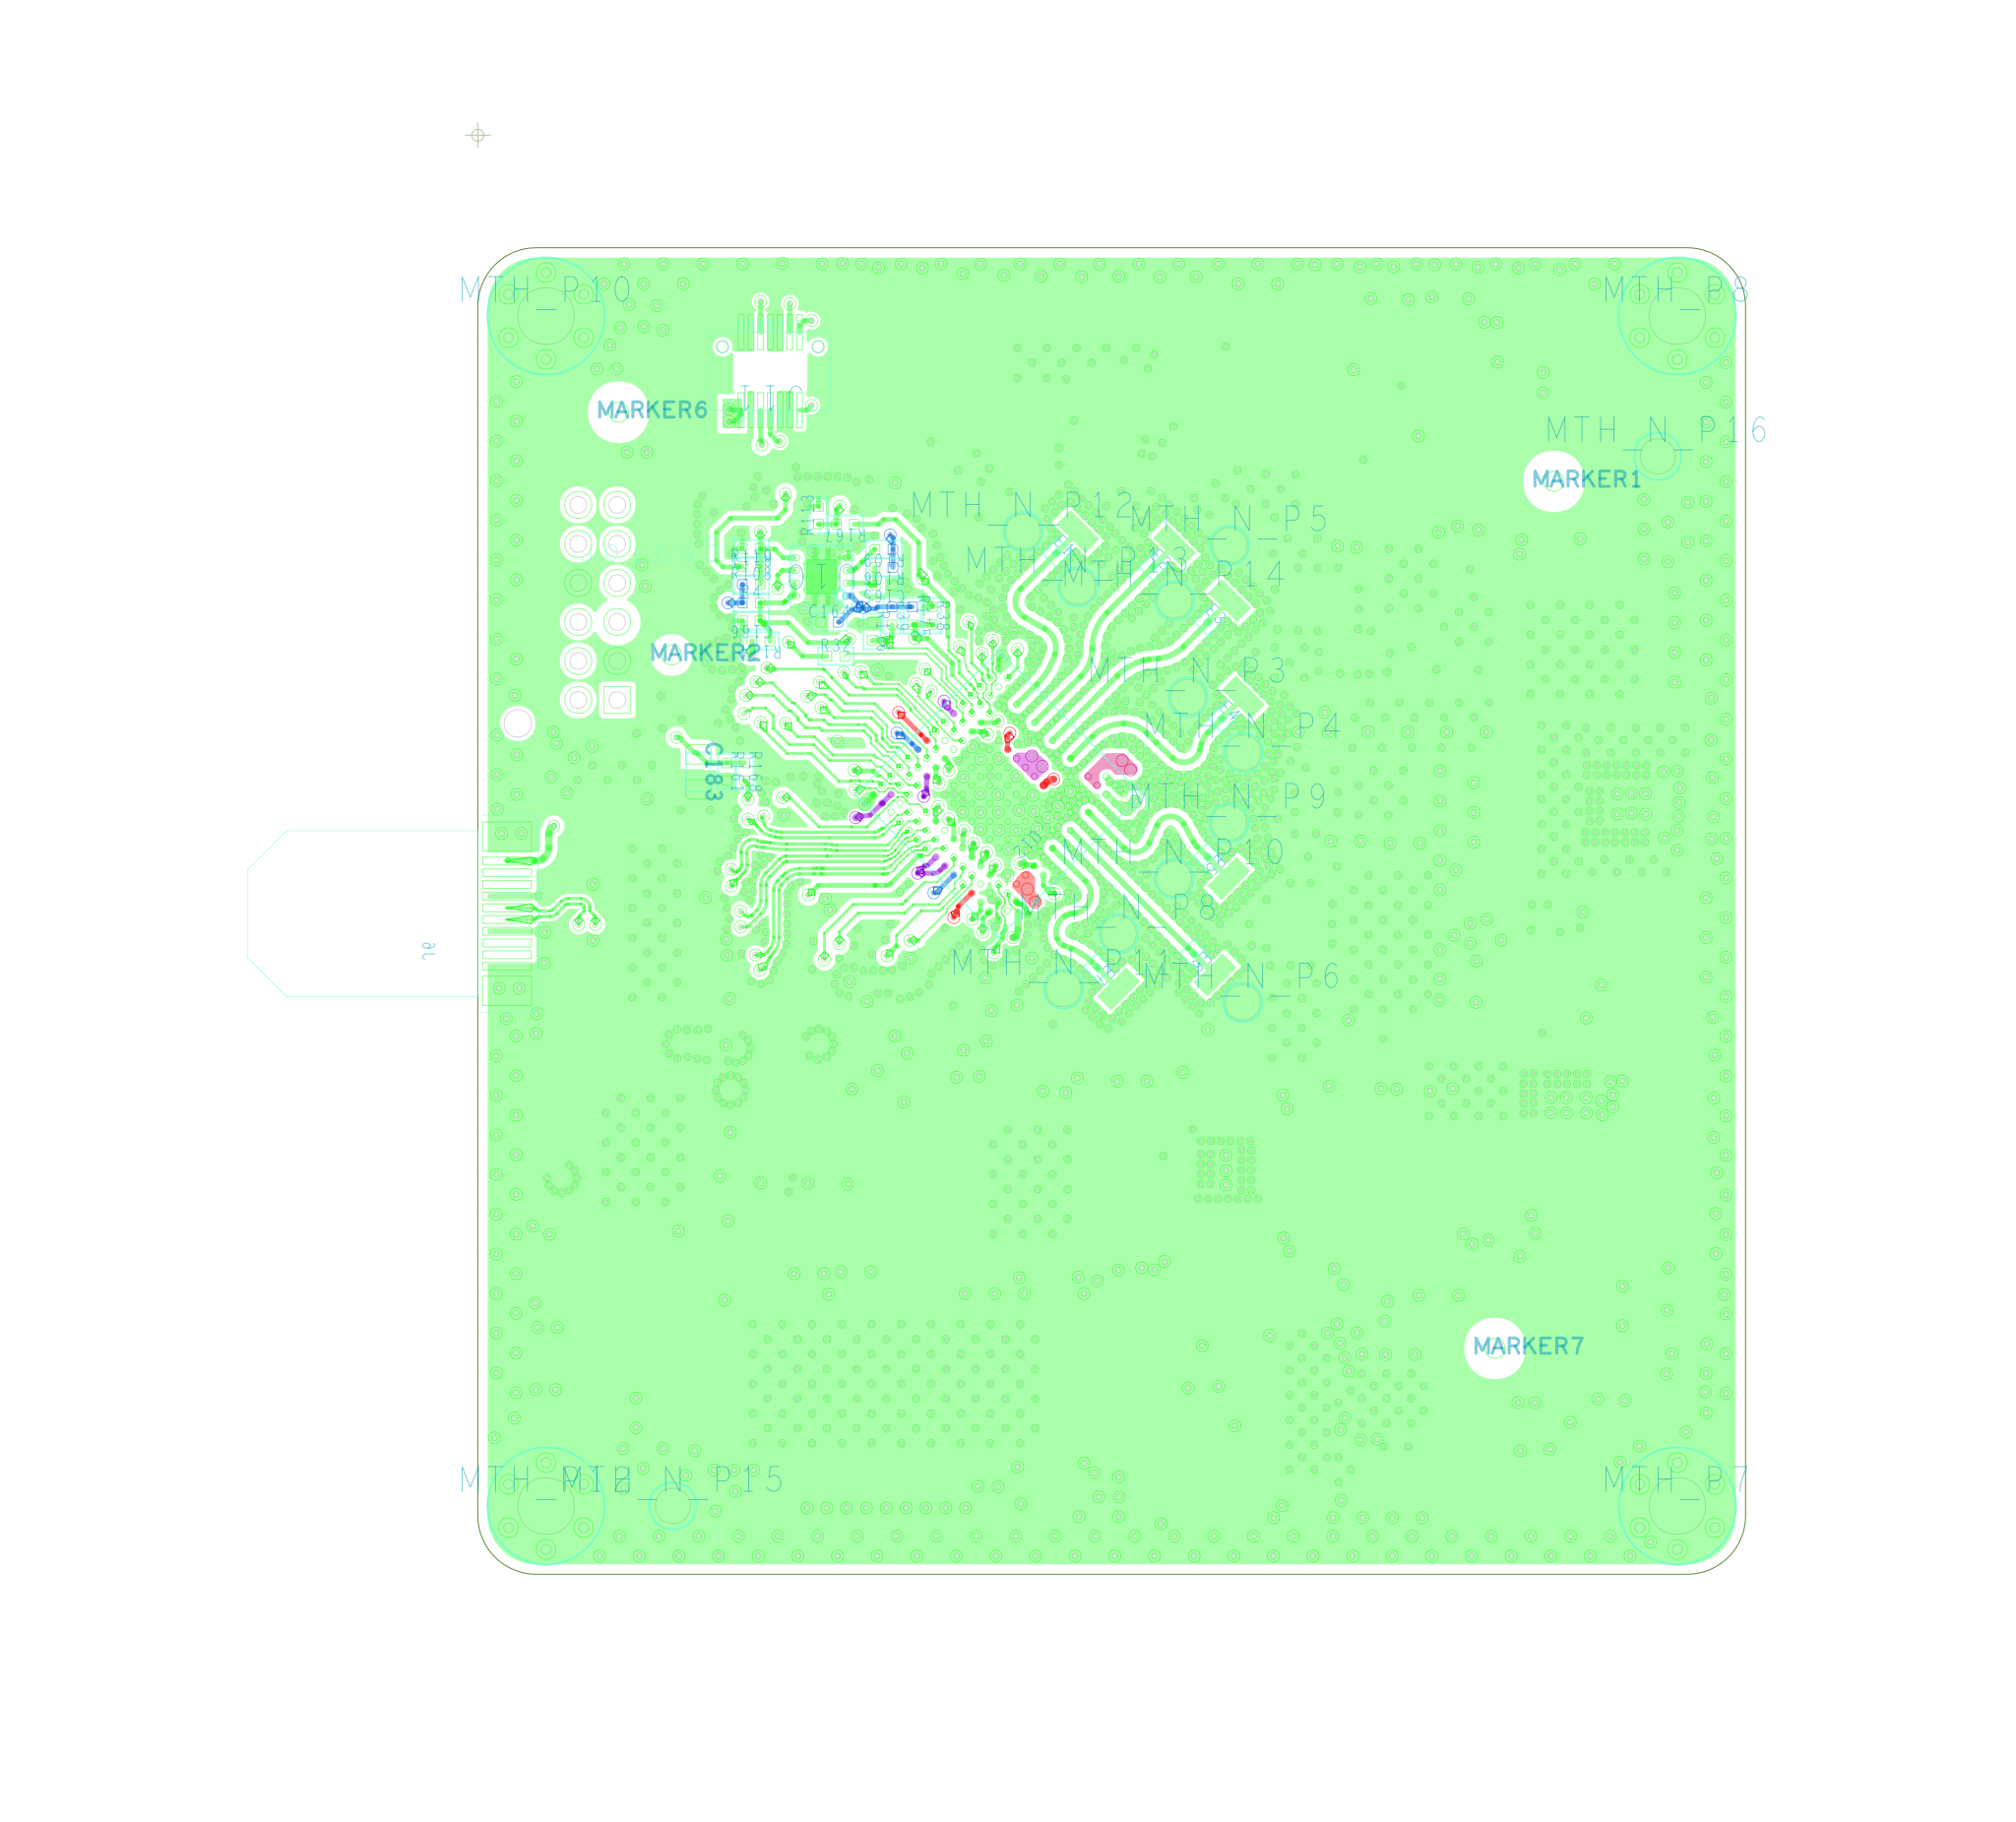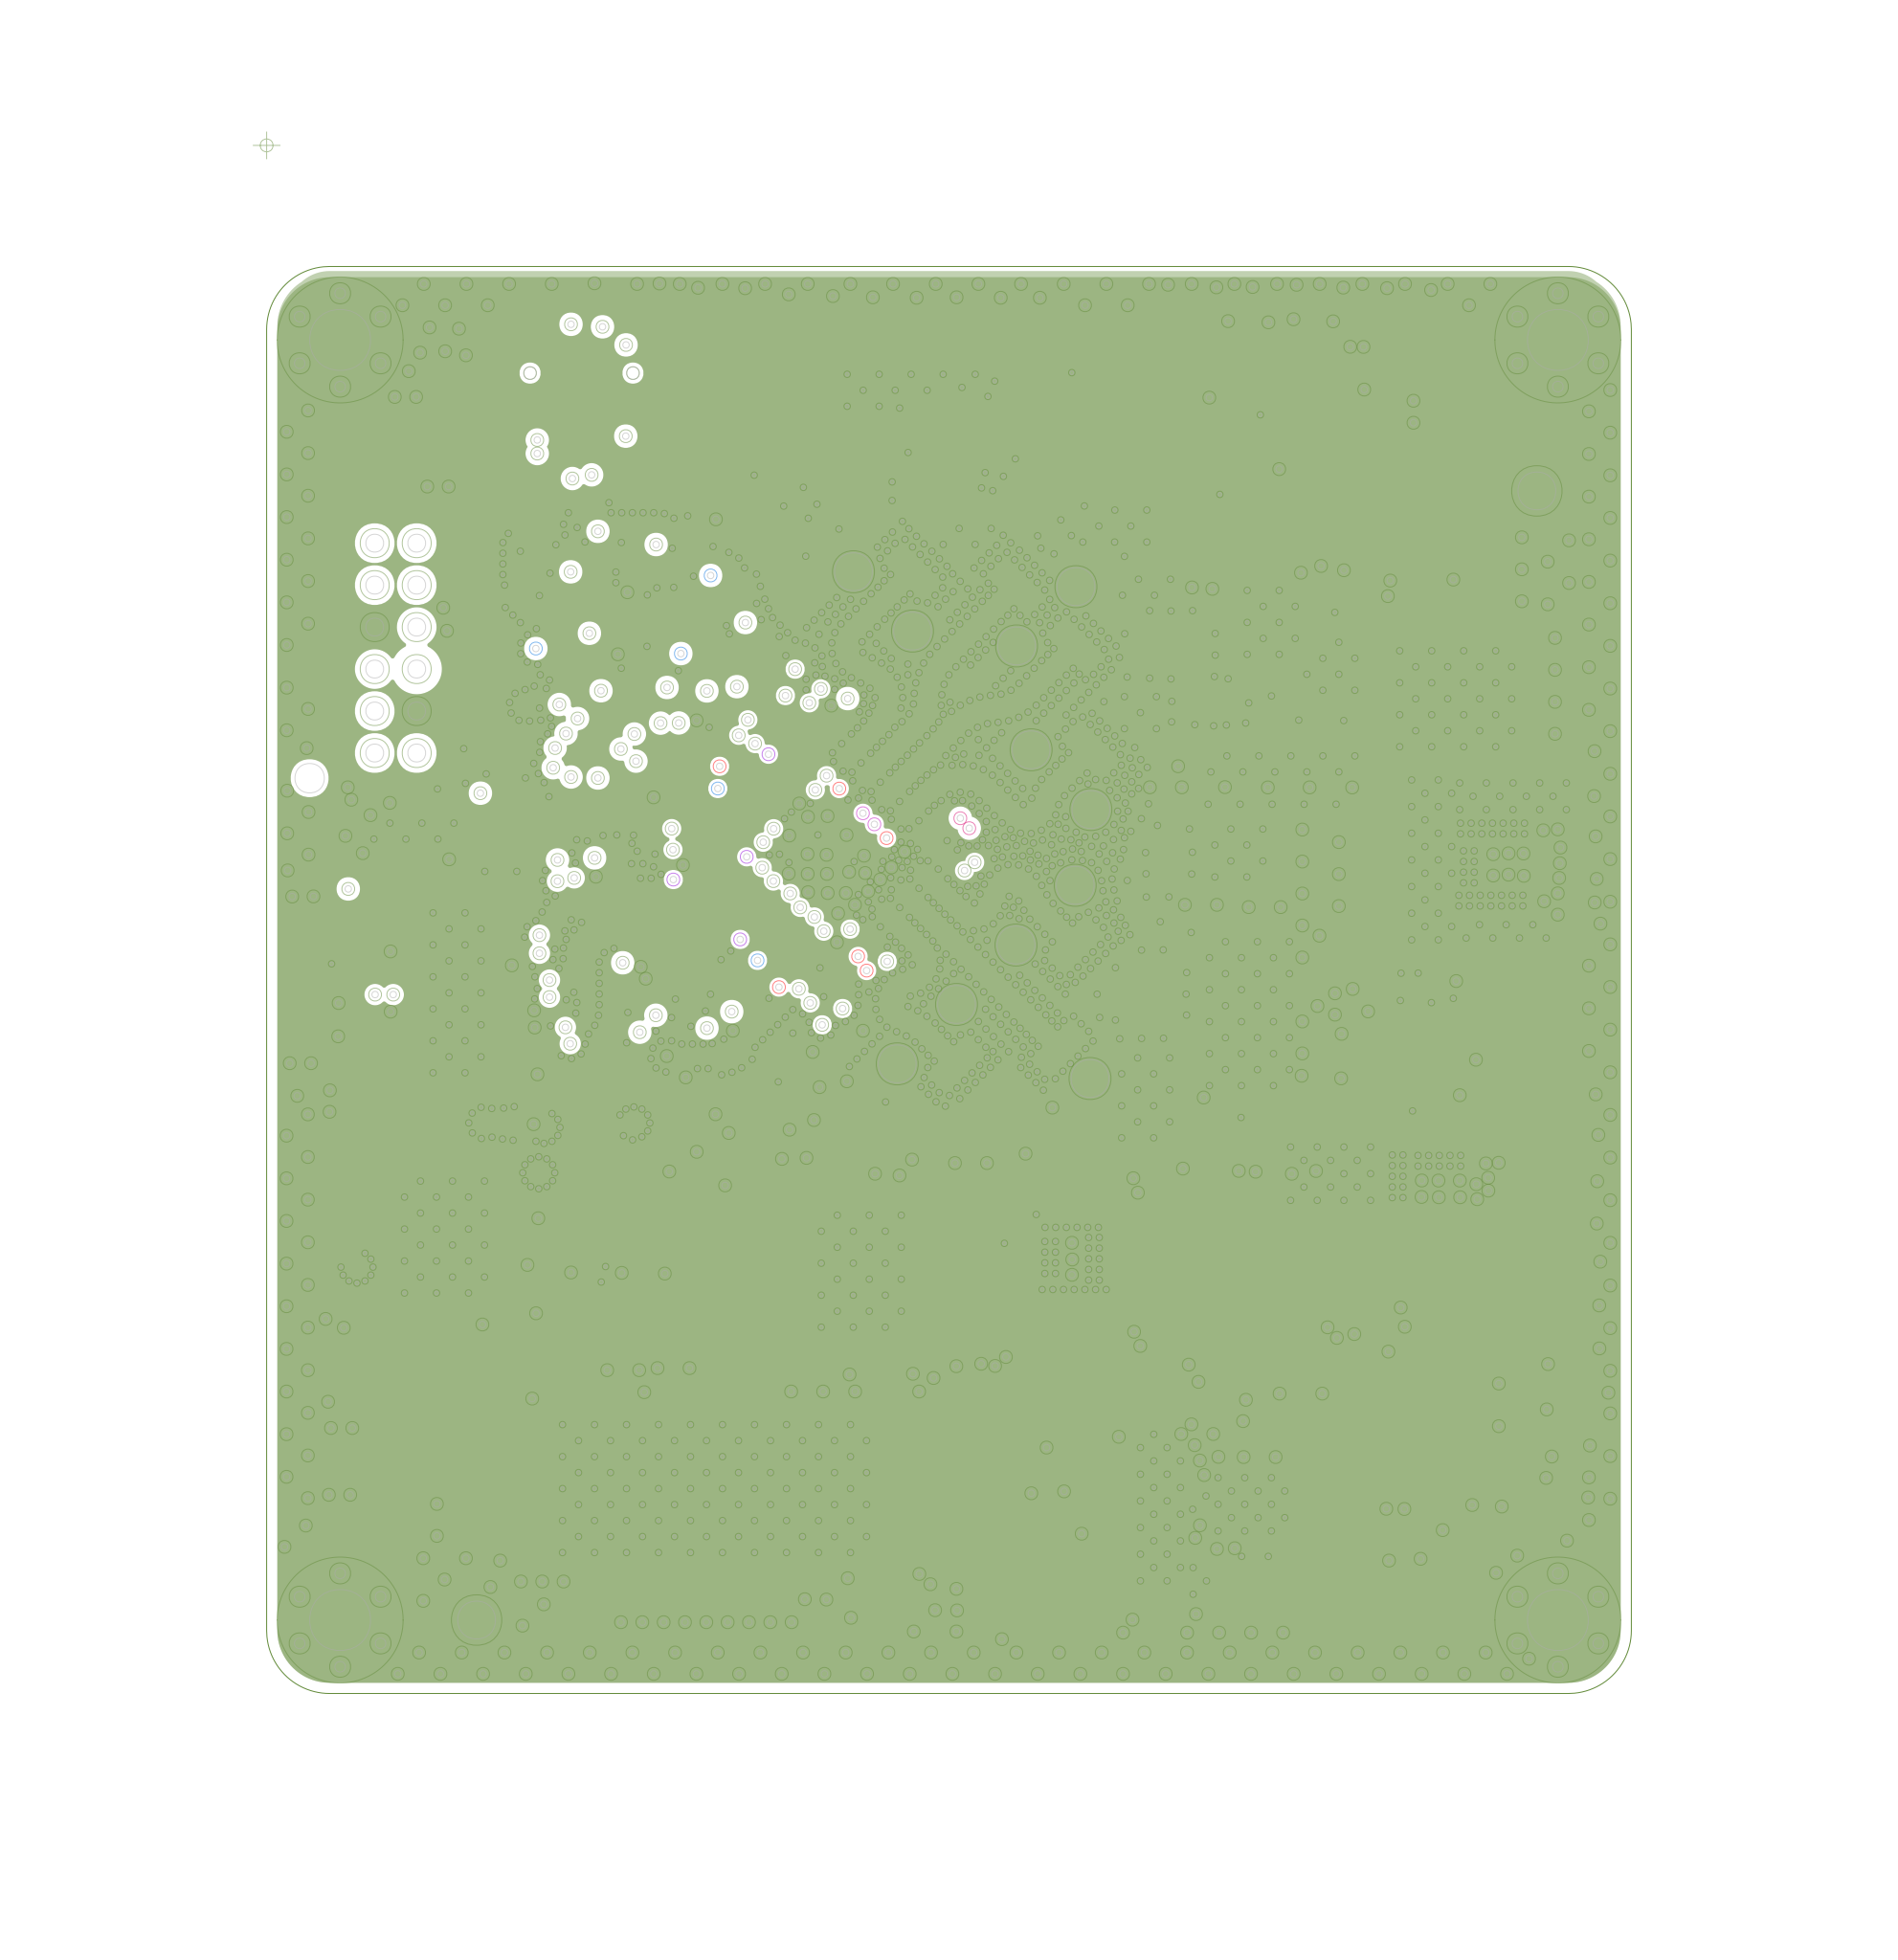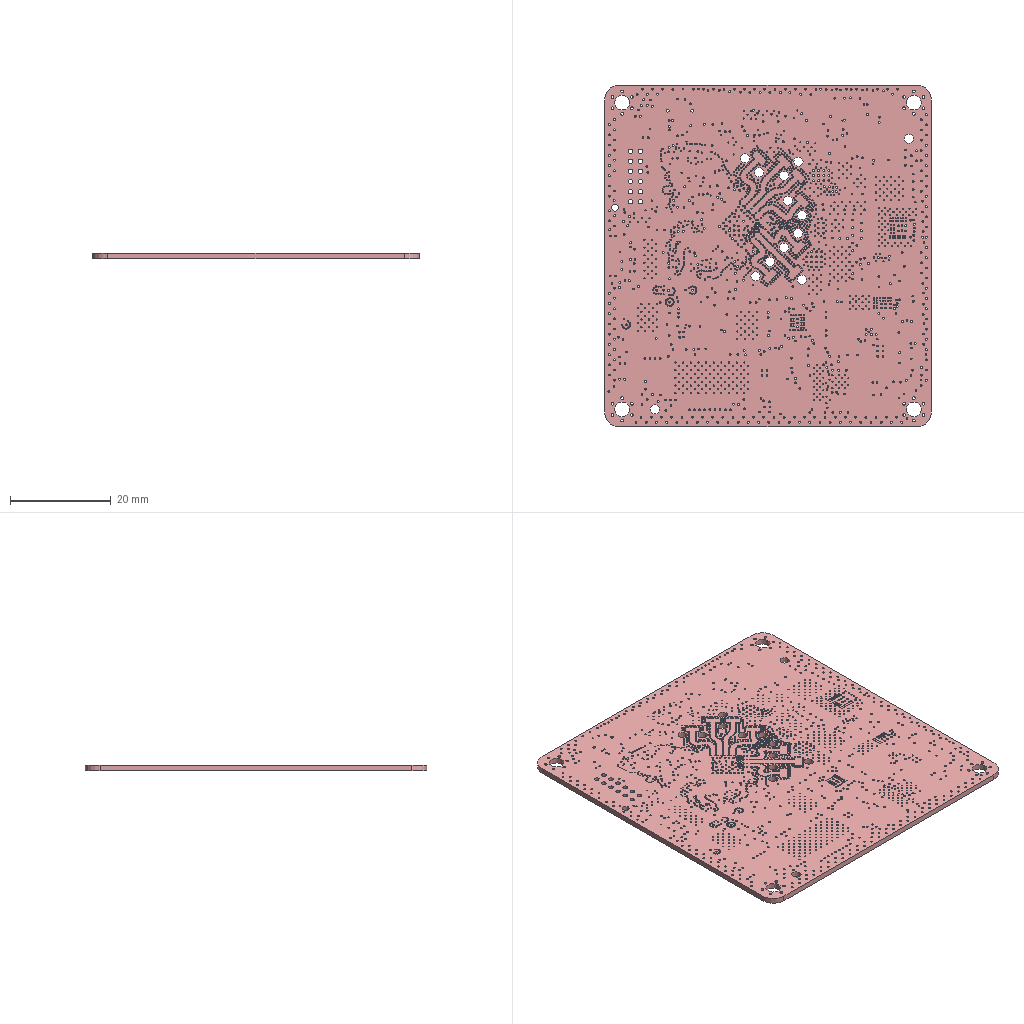Circuit board layout | Cadence Allegro | box 65 x 68 x 1.1 mm
Layer stack:
# Cadence Allegro layer stack of  (unit mm; from the constraint file cross-section; dielectric type: 0 not recorded (Allegro does not mark core vs prepreg), 3 surface material)
index,name,kind,layer,copper_thickness_mm,dielectric_type,dielectric_thickness_mm,dielectric_material,dielectric_constant
0,Top Surface,other,,,,,,
1,TOP,copper,TOP,0.0305,,,,
2,Dielectric1,dielectric,,,0,0.2032,FR-4,4.5
3,L2_GND,copper,L2_GND,0.0305,,,,
4,Dielectric2,dielectric,,,0,0.2032,FR-4,4.5
5,L3_SIGNAL,copper,L3_SIGNAL,0.0305,,,,
6,Dielectric3,dielectric,,,0,0.2032,FR-4,4.5
7,L4_POWER,copper,L4_POWER,0.0305,,,,
8,Dielectric4,dielectric,,,0,0.2032,FR-4,4.5
9,L5_GND,copper,L5_GND,0.0305,,,,
10,Dielectric5,dielectric,,,0,0.2032,FR-4,4.5
11,BOTTOM,copper,BOTTOM,0.0305,,,,
12,Bottom Surface,other,,,,,,
# drill layer pairs: low layer,high layer
drill_pair,TOP,BOTTOM
drill_pair,TOP,L2_GND
drill_pair,L3_SIGNAL,BOTTOM
Part placement:
REFDES,COMP_VALUE,SYM_NAME,SYM_X,SYM_Y,SYM_ROTATE,SYM_MIRROR
C1,10uf(NC),C0805,15.915,-52.198,90.000,YES
C2,10uf(NC),C0805,17.915,-52.198,90.000,YES
C3,10uf(NC),C0805,20.66,-37.958,315.000,YES
C4,10uf(NC),C0805,17.067,-56.426,90.000,YES
C6,10uf,C0805,30.967,-30.839,135.000,YES
C7,10uf(NC),C0805,47.332,-40.272,180.000,YES
C8,10uf,C0805,47.332,-38.272,180.000,YES
C9,10uf,C0805,47.332,-34.78,180.000,YES
C10,10uf,C0805,47.332,-32.78,180.000,YES
C11,10uf(NC),C0805,46.269,-21.899,270.000,YES
C12,10uf(NC),C0805,52.269,-21.899,270.000,YES
C13,10uf(NC),C0805,50.269,-21.899,270.000,YES
C14,10uf(NC),C0805,48.269,-21.899,270.000,YES
C15,10uf(NC),C0805,46.685,-29.053,90.000,YES
C16,10uf(NC),C0805,52.685,-29.053,90.000,YES
C17,10uf(NC),C0805,48.685,-29.053,90.000,YES
C18,10uf(NC),C0805,50.685,-29.053,90.000,YES
C19,.22uf,C0402,24.607,-38.207,225.000,YES
C20,.1uf,C0402,21.683,-36.883,315.000,YES
C21,2.2uf,C0603,16.96,-34.684,45.000,YES
C22,1uf,C0603,26.249,-39.694,315.000,YES
C23,.22uf,C0402,30.529,-32.465,135.000,YES
C24,.22uf,C0402,27.3,-29.488,315.000,YES
C25,.22uf,C0402,20.427,-28.78,315.000,YES
C26,.22uf,C0402,23.353,-40.764,45.000,YES
C27,.22uf,C0402,27.256,-38.958,315.000,YES
C28,.22uf,C0402,29.058,-37.834,225.000,YES
C29,.22uf,C0402,32.522,-34.13,45.000,YES
C30,.22uf,C0402,28.887,-36.578,225.000,YES
C31,10uf(NC),C0805,44.483,-38.019,270.000,YES
C32,10uf,C0805,28.452,-28.323,315.000,YES
C33,.22uf,C0402,28.216,-30.86,45.000,YES
C34,10uf,C0805,44.604,-29.053,90.000,YES
C35,.22uf,C0402,31.861,-33.449,45.000,YES
C36,2.2uf,C0603,20.921,-31.978,135.000,YES
C37,.22uf,C0402,22.251,-31.553,135.000,YES
C38,1uf,C0603,31.504,-37.042,225.000,YES
C39,.22uf,C0402,24.207,-27.453,225.000,YES
C40,10000pf,C0402,24.88,-28.116,225.000,YES
C41,.22uf,C0402,23.17,-36.898,315.000,YES
C42,10uf(NC),C0805,47.332,-42.272,180.000,YES
C43,.1uf,C0402,15.012,-33.406,225.000,YES
C44,4.7pf,C0402,20.689,-43.422,45.000,YES
C45,4.7pf,C0402,24.624,-46.029,45.000,YES
C46,.1uf,C0402,23.59,-16.301,90.000,YES
C47,10000pf,C0402,41.102,-68.934,90.000,YES
C48,.1uf,C0805,42.562,-69.266,90.000,YES
C49,.1uf,C0805,42.373,-59.059,180.000,YES
C50,.1uf,C0805,39.642,-69.266,90.000,YES
C51,10000pf,C0402,42.373,-60.519,180.000,YES
C55,.47uf,C0603,38.805,-60.356,0.000,YES
C59,.1uf,C0402,38.005,-62.512,270.000,YES
C71,10uf,C1210,35.797,-69.415,0.000,YES
C72,10uf,C1210,35.047,-64.652,270.000,YES
C73,10uf,C1210,38.005,-58.006,0.000,YES
C80,22uf,C1210,53.352,-38.271,0.000,YES
C81,22uf,C1210,58.673,-27.745,180.000,YES
C82,22uf,C1210,58.673,-24.545,180.000,YES
C83,10uf,C0805,52.163,-46.069,270.000,YES
C84,10uf,C0805,50.127,-46.069,270.000,YES
C86,10uf,C0805,55.397,-54.84,90.000,YES
C87,10uf,C0805,57.409,-54.839,90.000,YES
C101,10uf,C0805,42.941,-56.159,90.000,YES
C102,10uf,C0805,33.785,-50.53,270.000,YES
C103,10uf,C0805,42.889,-50.53,270.000,YES
C104,10uf,C0805,33.788,-56.159,90.000,YES
C105,22uf,C1210,25.931,-56.52,90.000,YES
C108,22uf,C1210,25.931,-51.087,270.000,YES
C111,22uf,C1210,50.279,-56.538,90.000,YES
C113,22uf,C1210,50.325,-51.408,270.000,YES
C115,22uf,C1210,58.356,-61.82,180.000,YES
C116,22uf,C1210,54.139,-64.634,90.000,YES
C117,22uf,C1210,58.373,-58.547,180.000,YES
C124,.1uf,C0402,57.485,-30.822,180.000,YES
C125,.1uf,C0402,57.018,-38.677,90.000,YES
C126,.1uf,C0402,54.772,-41.109,0.000,YES
C127,10000pf,C0402,58.889,-30.372,90.000,YES
C128,10uf,C0805,53.923,-42.608,0.000,YES
C129,.1uf,C0402,59.487,-37.775,180.000,YES
C138,.22uf,C0402,28.141,-57.3,90.000,YES
C139,.22uf,C0402,28.15,-49.706,270.000,YES
C140,.22uf,C0402,48.016,-57.212,90.000,YES
C141,.22uf,C0402,47.989,-49.675,270.000,YES
C142,.22uf,C0402,36.725,-49.102,0.000,YES
C143,390PF,C0402,31.348,-57.722,0.000,YES
C144,390PF,C0402,31.348,-49.229,0.000,YES
C145,390PF,C0402,45.148,-57.712,180.000,YES
C146,390PF,C0402,45.15,-49.154,180.000,YES
C147,.1uf,C0402,53.918,-54.158,90.000,YES
C148,.1uf,C0402,51.212,-48.447,0.000,YES
C149,.47uf,C0603,59.05,-50.013,270.000,YES
C151,.1uf,C0805,7.432,-62.35,90.000,YES
C152,47uF,CAPAE630X800N,29.395,-65.323,90.000,YES
C153,.1uf,C0805,24.165,-68.37,90.000,YES
C154,4.7uF,C0805,21.996,-68.37,90.000,YES
C155,.1uf,C0805,12.536,-66.392,90.000,YES
C156,1uf,C0805,14.705,-66.392,90.000,YES
C157,.1uf,C0805,17.657,-68.37,90.000,YES
C158,1uf,C0805,19.826,-68.37,90.000,YES
C161,.1uf,C0805,4.563,-62.605,0.000,YES
C163,.47uf,C0603,53.913,-45.869,270.000,YES
C164,.1uf,C0402,18.032,-24.964,0.000,NO
C165,.1uf,C0402,20.822,-23.075,180.000,NO
C166,.1uf,C0402,14.018,-24.896,180.000,NO
C167,.1uf,C0402,13.748,-56.212,90.000,YES
C168,.1uf,C0402,4.29,-57.58,270.000,YES
C169,.1uf,C0402,61.098,-45.616,180.000,YES
C172,.1uf,C0402,33.697,-16.241,0.000,YES
C173,.1uf,C0402,39.01,-16.157,0.000,YES
C174,.1uf,C0402,36.46,-16.143,0.000,YES
C175,4700pf,C0603,9.991,-38.982,180.000,YES
C176,100pf,C0603,11.327,-35.829,90.000,YES
C177,100pf,C0603,6.227,-35.829,90.000,YES
C178,.1uf,C0402,18.268,-35.087,45.000,YES
C179,.22uf,C0402,49.814,-60.71,0.000,YES
C180,4.7uF,C0805,35.197,-61.302,0.000,YES
C182,.1uf,C0805,9.12,-12.46,270.000,YES
C183,.1uf,C0805,11.301,-32.639,270.000,NO
C184,.1uf,C0402,18.552,-56.685,90.000,YES
C185,.1uf,C0402,37.191,-64.461,270.000,YES
D2,3A,SMB,12.125,-61.86,0.000,YES
D9,LED,LED0603,46.346,-69.477,180.000,YES
D12,SM24CANB-02HTG,SOT23,8.777,-35.829,180.000,YES
E1,ANTENNA,ANTENNA,29.679,-21.408,315.000,NO
E2,ANTENNA,ANTENNA,34.629,-22.115,315.000,NO
E3,ANTENNA,ANTENNA,37.457,-24.944,315.000,NO
E4,ANTENNA,ANTENNA,38.164,-29.893,315.000,NO
E5,ANTENNA,ANTENNA,37.423,-37.018,225.000,NO
E6,ANTENNA,ANTENNA,36.715,-41.968,225.000,NO
E7,ANTENNA,ANTENNA,31.765,-42.675,225.000,NO
J6,LVDS,LVDS,1.5,-43.86,270.000,YES
J9,6,TST6X254,43.243,-9.705,270.000,YES
J10,5016451220,5016451220,7.148,-28.954,270.000,YES
J11,2x7,CON2X7X200,14.997,-12.1,180.000,NO
J12,6,TST6X254,25.18,-9.658,90.000,YES
L1,120R,L0603,53.687,-24.492,0.000,YES
L2,100nH,NLCV32T-R10M-EFRD,47.09,-45.804,270.000,YES
L3,120R,L0603,53.653,-26.325,0.000,YES
L4,120R,L0603,47.09,-45.804,270.000,YES
L5,120R,L0603,21.644,-51.942,0.000,YES
L6,100nH,NLCV32T-R10M-EFRD,21.601,-51.974,0.000,YES
L7,120R,L0603,21.58,-56.288,0.000,YES
L8,100nH,NLCV32T-R10M-EFRD,21.579,-56.23,0.000,YES
L9,2.2uH,SPM5030,48.855,-64.617,180.000,YES
L14,120R(NC),L0603,54.947,-34.941,270.000,YES
L15,120R(NC),L0603,53.446,-34.941,270.000,YES
L16,0.47uH,L2520,29.658,-54.971,0.000,YES
L17,0.47uH,L2520,46.476,-54.917,180.000,YES
L18,0.47uH,L2520,29.682,-52.024,0.000,YES
L19,0.47uH,L2520,46.476,-51.971,180.000,YES
L21,600R,L0805,17.109,-64.892,270.000,YES
L22,10uH,SPM5030,21.622,-63.282,180.000,YES
L23,120R(NC),L0603,52.957,-50.145,270.000,YES
L24,51uH,CM320X450X150-4N,7.287,-50.113,180.000,YES
L25,600R(NC),L0805,21.618,-63.252,180.000,YES
MARKER1,D3,FIDMS0,55.168,-17.75,0.000,NO
MARKER2,D2,FIDMS1,9.934,-26.647,0.000,NO
MARKER3,D2,FIDMS1,42.03,-27.204,0.000,YES
MARKER4,D3,FIDMS0,5.956,-65.764,0.000,YES
MARKER5,D3,FIDMS0,5.501,-14.077,0.000,YES
MARKER6,D3,FIDMS0,7.215,-14.2,0.000,NO
MARKER7,D3,FIDMS0,52.148,-62.192,0.000,NO
MARKER8,D3,FIDMS0,56.674,-69.361,0.000,YES
MTH_N_P3,D1.6plated_NV,MTGP200H160P,36.412,-28.802,0.000,NO
MTH_N_P4,D1.6plated_NV,MTGP200H160P,39.257,-31.648,0.000,NO
MTH_N_P5,D1.6plated_NV,MTGP200H160P,38.547,-21.027,0.000,NO
MTH_N_P6,D1.6plated_NV,MTGP200H160P,39.217,-44.465,0.000,NO
MTH_N_P8,D1.6plated_NV,MTGP200H160P,32.858,-40.936,0.000,NO
MTH_N_P9,D1.6plated_NV,MTGP200H160P,38.511,-35.258,0.000,NO
MTH_N_P10,D1.6plated_NV,MTGP200H160P,35.691,-38.106,0.000,NO
MTH_N_P11,D1.6plated_NV,MTGP200H160P,30.034,-43.767,0.000,NO
MTH_N_P12,D1.6plated_NV,MTGP200H160P,27.95,-20.317,0.000,NO
MTH_N_P13,D1.6plated_NV,MTGP200H160P,30.762,-23.143,0.000,NO
MTH_N_P14,D1.6plated_NV,MTGP200H160P,35.718,-23.853,0.000,NO
MTH_N_P15,D1.8plated_NV,MTGP240H180P,10,-70.271,0.000,NO
MTH_N_P16,D1.8plated_NV,MTGP240H180P,60.5,-16.465,0.000,NO
MTH_P7,M2.5,MTGP600H290V6P,61.5,-70.271,0.000,NO
MTH_P8,M2.5,MTGP600H290V6P,61.5,-9.271,0.000,NO
MTH_P10,M2.5,MTGP600H290V6P,3.5,-9.271,0.000,NO
MTH_P12,M2.5,MTGP600H290V6P,3.5,-70.271,0.000,NO
R1,0R(NC),R0603,54.495,-29.053,270.000,YES
R4,4.7k,R0402,14.018,-23.976,0.000,NO
R6,4.7k,R0402,20.369,-33.434,135.000,YES
R7,4.7k,R0402,19.755,-29.452,315.000,YES
R8,4.7k,R0402,24.498,-29.911,225.000,YES
R9,1k,R0402,45.352,-15.294,270.000,YES
R10,1k,R0402,46.482,-15.271,270.000,YES
R11,1k,R0402,21.291,-12.128,270.000,YES
R12,1k,R0402,26.449,-12.777,270.000,YES
R13,1k,R0402,23.979,-12.163,270.000,YES
R14,1k,R0402,19.848,-12.149,270.000,YES
R15,4.7k,R0402,25.117,-12.97,90.000,YES
R18,10k,R0402,23.933,-36.159,315.000,YES
R19,0R,R0402,45.596,-59.141,270.000,YES
R20,0R,R0402,17.388,-44.892,270.000,YES
R21,0R,R0402,16.468,-44.892,270.000,YES
R23,10k,R0402,16.278,-48.317,270.000,YES
R24,10k,R0402,15.358,-48.317,270.000,YES
R25,1k,R0402,16.875,-40.439,225.000,YES
R26,1k,R0402,17.55,-41.118,225.000,YES
R32,1k,R0402,18.357,-26.716,0.000,NO
R36,1k,R0402,15.244,-39.364,225.000,YES
R38,10k,R0402,23.301,-24.637,270.000,NO
R39,10k(NC),R0402,21.238,-24.643,270.000,NO
R42,10k,R0402,42.529,-15.294,90.000,YES
R43,1k,R0402,43.515,-15.29,90.000,YES
R44,0R,R0402,24.414,-41.271,225.000,YES
R45,1k,R0402,11.444,-47.789,270.000,YES
R46,1k,R0402,10.524,-47.789,270.000,YES
R47,1k,R0402,18.377,-36.672,225.000,YES
R49,10k,R0402,21.433,-14.402,0.000,YES
R50,10k,R0402,13.76,-24.363,90.000,YES
R51,10k,R0402,20.859,-24.271,180.000,YES
R52,10k,R0402,37.458,-65.936,180.000,YES
R53,1k,R0603,49.862,-69.477,0.000,YES
R76,10k,R0402,17.984,-32.719,315.000,YES
R80,12k,R0402,59.809,-30.362,90.000,YES
R81,48.7k,R0402,60.773,-30.362,270.000,YES
R86,3.83R,R0402,31.348,-56.802,180.000,YES
R87,3.83R,R0402,31.348,-50.175,180.000,YES
R88,3.83R,R0402,45.16,-56.762,0.000,YES
R89,3.83R,R0402,45.16,-50.096,0.000,YES
R90,1k,R0402,59.228,-55.867,270.000,YES
R91,1.96k,R0402,60.148,-55.856,90.000,YES
R92,10k,R0402,60.348,-50.115,90.000,YES
R93,4.99k,R0402,60.148,-53.985,270.000,YES
R94,10k,R0402,61.408,-50.126,90.000,YES
R95,10k,R0402,61.068,-55.836,270.000,YES
R96,4.99k,R0402,59.228,-53.985,270.000,YES
R97,4.99k(NC),R0402,61.068,-53.985,270.000,YES
R103,12.7k,R0402,55.123,-45.239,270.000,YES
R104,10k,R0402,57.248,-46.488,0.000,YES
R105,0R(NC),R0603,3.937,-47.441,90.000,YES
R106,10k(NC),R0402,20.822,-22.155,180.000,NO
R108,10k,R0402,14.018,-23.034,0.000,NO
R109,10k,R0402,20.822,-21.235,180.000,NO
R110,1k,R0402,14.018,-22.114,0.000,NO
R111,0R(NC),R0402,14.018,-21.194,180.000,NO
R112,0R,R0402,24.763,-22.783,270.000,YES
R113,10k,R0402,17.463,-19.487,90.000,NO
R116,1k,R0402,61.088,-43.775,0.000,YES
R118,47k,R0402,61.088,-42.855,180.000,YES
R119,1k,R0402,61.088,-44.695,0.000,YES
R127,1k,R0402,33.687,-15.192,180.000,YES
R130,1k,R0402,39.025,-15.144,180.000,YES
R133,1k,R0402,36.452,-15.111,180.000,YES
R141,0R(NC),R0402,4.389,-50.23,90.000,YES
R142,62R,R1206,9.005,-42.141,270.000,YES
R143,62R,R1206,11.305,-42.141,270.000,YES
R144,0R(NC),R0402,10.147,-50.113,90.000,YES
R150,10k,R0402,61.765,-30.362,270.000,YES
R161,10k,R0402,12.761,-32.639,270.000,NO
R167,10k,R0402,18.843,-19.947,180.000,NO
R168,10k,R0402,13.681,-32.639,270.000,NO
R169,10k,R0402,22.531,-39.959,45.000,YES
R170,33R,R0402,11.312,-17.99,180.000,YES
R171,33R,R0402,11.328,-19.048,180.000,YES
R172,33R,R0402,11.314,-16.913,180.000,YES
R173,33R,R0402,20.691,-41.291,45.000,YES
R174,0R,R0402,14.514,-25.931,180.000,NO
R175,10k(NC),R0402,22.28,-24.641,270.000,NO
R176,10k,R0402,20.216,-25.445,270.000,NO
R177,0R,R0402,60.891,-51.77,0.000,YES
R178,10k,R0402,39.029,-14.111,180.000,YES
R179,10k,R0402,33.675,-14.159,180.000,YES
R180,10k,R0402,36.443,-14.087,180.000,YES
R181,1k,R0402,29.855,-14.494,90.000,YES
R182,1k,R0402,28.67,-14.505,90.000,YES
R183,1k,R0402,30.888,-14.491,90.000,YES
R184,0R(NC),R0805,14.954,-12.849,90.000,YES
TP1,33mil,TPAD_33MIL,10.783,-65.298,0.000,YES
TP2,33mil,TPAD_33MIL,15.238,-68.847,0.000,YES
TP3,33mil,TPAD_33MIL,44.242,-68.303,90.000,YES
TP4,33mil,TPAD_33MIL,6.813,-59.846,270.000,YES
TP6,33mil,TPAD_33MIL,16.82,-59.152,90.000,YES
TP9,33mil,TPAD_33MIL,52.171,-69.375,180.000,YES
TP10,33mil,TPAD_33MIL,60.171,-64.584,90.000,YES
TP14,33mil,TPAD_33MIL,29.278,-57.006,90.000,YES
TP15,33mil,TPAD_33MIL,23.131,-49.619,90.000,YES
TP16,33mil,TPAD_33MIL,52.585,-54.34,270.000,YES
TP17,33mil,TPAD_33MIL,52.73,-52.531,270.000,YES
TP18,33mil,TPAD_33MIL,29.482,-58.358,270.000,YES
TP19,33mil,TPAD_33MIL,29.692,-49.985,270.000,YES
TP20,33mil,TPAD_33MIL,46.745,-56.965,270.000,YES
TP21,33mil,TPAD_33MIL,46.747,-49.936,270.000,YES
TP29,33mil,TPAD_33MIL,55.488,-47.142,270.000,YES
TP30,33mil,TPAD_33MIL,55.917,-32.164,90.000,YES
TP31,33mil,TPAD_33MIL,33.389,-27.349,0.000,YES
TP32,33mil,TPAD_33MIL,50.131,-26.48,0.000,YES
TP33,33mil,TPAD_33MIL,29.309,-40.092,0.000,YES
TP34,33mil,TPAD_33MIL,20.559,-49.552,270.000,YES
TP35,33mil,TPAD_33MIL,15.038,-57.398,270.000,YES
TP37,33mil,TPAD_33MIL,27.321,-42.838,135.000,YES
TP41,33mil,TPAD_33MIL,39.399,-17.308,270.000,YES
TP42,33mil,TPAD_33MIL,36.481,-17.541,180.000,YES
TP44,33mil,TPAD_33MIL,61.286,-41.084,180.000,YES
TP47,33mil,TPAD_33MIL,13.634,-27.631,0.000,YES
TP48,33mil,TPAD_33MIL,14.898,-24.947,90.000,YES
TP49,33mil,TPAD_33MIL,15.626,-30.12,0.000,YES
TP50,33mil,TPAD_33MIL,13.387,-30.018,90.000,YES
TP51,33mil,TPAD_33MIL,11.982,-27.128,0.000,YES
TP52,33mil,TPAD_33MIL,16.744,-28.81,90.000,YES
TP53,33mil,TPAD_33MIL,13.644,-58.32,270.000,YES
TP56,33mil,TPAD_33MIL,13.406,-53.858,270.000,YES
TP57,33mil,TPAD_33MIL,4.303,-54.332,90.000,YES
TP58,33mil,TPAD_33MIL,8.591,-32.827,0.000,YES
TP59,33mil,TPAD_33MIL,7.037,-32.841,0.000,YES
TP65,33mil,TPAD_33MIL,19.457,-25.927,180.000,YES
TP66,33mil,TPAD_33MIL,15.925,-24.969,180.000,YES
TP68,33mil,TPAD_33MIL,14.401,-20.16,180.000,YES
TP79,33mil,TPAD_33MIL,22.778,-12.309,90.000,YES
TP80,33mil,TPAD_33MIL,25.433,-24.877,90.000,YES
TP81,33mil,TPAD_33MIL,45.297,-16.881,180.000,YES
TP82,33mil,TPAD_33MIL,46.537,-13.227,180.000,YES
TP83,33mil,TPAD_33MIL,45.089,-13.264,270.000,YES
TP84,33mil,TPAD_33MIL,25.726,-28.887,90.000,YES
TP86,33mil,TPAD_33MIL,21.743,-34.395,90.000,YES
TP90,33mil,TPAD_33MIL,44.618,-33.337,90.000,YES
TP91,33mil,TPAD_33MIL,29.929,-38.806,90.000,YES
TP94,33mil,TPAD_33MIL,43.487,-16.947,90.000,YES
TP95,33mil,TPAD_33MIL,18.57,-28.359,0.000,YES
TP100,33mil,TPAD_33MIL,20.759,-25.841,90.000,YES
TP101,33mil,TPAD_33MIL,21.874,-25.405,90.000,YES
TP102,33mil,TPAD_33MIL,16.114,-46.539,0.000,YES
TP103,33mil,TPAD_33MIL,17.48,-46.601,90.000,YES
TP104,33mil,TPAD_33MIL,11.651,-45.497,270.000,YES
TP108,33mil,TPAD_33MIL,23.476,-21.7,0.000,YES
TP109,33mil,TPAD_33MIL,13.417,-34.157,0.000,YES
TP118,debug,TST1,6.779,-44.405,0.000,YES
TP119,debug,TST1,16.308,-37.011,0.000,YES
TP120,debug,TST1,11.809,-50.456,180.000,YES
TP121,33mil,TPAD_33MIL,33.279,-12.828,0.000,YES
TP122,33mil,TPAD_33MIL,35.967,-12.815,180.000,YES
TP123,33mil,TPAD_33MIL,38.662,-12.87,0.000,YES
TP124,33mil,TPAD_33MIL,28.628,-12.84,90.000,YES
TP125,33mil,TPAD_33MIL,30.002,-12.876,90.000,YES
TP127,33mil,TPAD_33MIL,31.358,-12.81,90.000,YES
U2,IS25LP032D-JNLA3,SOIC127P600X175-8N,19.934,-19.108,270.000,YES
U3,LM536255QRNLRQ1,RNL0022A,41.411,-64.192,90.000,YES
U5,LP87524BRNFRQ1,RNF0026C,38.371,-53.121,270.000,YES
U7,TPS7A5301QRGRRQ1,RGR0020A,59.154,-34.284,90.000,YES
U9,TPS7A8101QDRBRQ1,DRB0008A,56.32,-49.757,90.000,YES
U10,TPS3851G33SQDRBRQ1,DRB0008A,17.615,-22.639,180.000,NO
U11,TJA1044GT/3Z,SOIC127P600X175-8N,8.773,-56.255,0.000,YES
U12,IWR1843AQGABL,ABL0161B,26.7,-33.792,225.000,NO
Y1,40MHz,OSCCC250X320X85-4N,22.89,-44.449,315.000,YES
Pad and via stacks:
# Allegro (Cadence) via spans and padstacks; design units: ("millimeters" 4 10000)
# via spans: padstack,start_layer,end_layer,net_example,count
BBVIA1_2_NO,ETCH/TOP,ETCH/L2_GND,GND,79
OPENVIA24D12_3-6_DBFIX2,ETCH/L3_SIGNAL,ETCH/BOTTOM,3V3_AR1,53
OPENVIA24D12_3-6,ETCH/L3_SIGNAL,ETCH/BOTTOM,LVDS_TXP0_AR1,110
BBVIA1_2,ETCH/TOP,ETCH/L2_GND,GND,1453
OPENVIA24D12,ETCH/TOP,ETCH/BOTTOM,GND,607
OPENVIA24D12_3-6_DBFIX1,ETCH/L3_SIGNAL,ETCH/BOTTOM,5V,28
# Allegro padstack definitions: name,start_layer,end_layer,drill,plating,holeType,type
RR165_40,"ETCH/TOP","ETCH/TOP",0.0,"NON_PLATED","none","smd"
RR315_40,"ETCH/TOP","ETCH/TOP",0.0,"NON_PLATED","none","smd"
RR100_40,"ETCH/TOP","ETCH/TOP",0.0,"NON_PLATED","none","smd"
RR75_25,"ETCH/TOP","ETCH/TOP",0.0,"NON_PLATED","none","smd"
RR60_25,"ETCH/TOP","ETCH/TOP",0.0,"NON_PLATED","none","smd"
RR60_40,"ETCH/TOP","ETCH/TOP",0.0,"NON_PLATED","none","smd"
R60_25,"ETCH/TOP","ETCH/TOP",0.0,"NON_PLATED","none","smd"
R224_66,"ETCH/TOP","ETCH/TOP",0.0,"NON_PLATED","none","smd"
R182_25,"ETCH/TOP","ETCH/TOP",0.0,"NON_PLATED","none","smd"
R77_5_40,"ETCH/TOP","ETCH/TOP",0.0,"NON_PLATED","none","smd"
D90_30,"ETCH/TOP","ETCH/TOP",0.0,"NON_PLATED","none","smd"
S215,"ETCH/TOP","ETCH/TOP",0.0,"NON_PLATED","none","smd"
R90_50,"ETCH/TOP","ETCH/TOP",0.0,"PLATED","none","smd"
R315_220,"ETCH/TOP","ETCH/TOP",0.0,"PLATED","none","smd"
R340_260,"ETCH/TOP","ETCH/TOP",0.0,"PLATED","none","smd"
R145_95,"ETCH/TOP","ETCH/TOP",0.0,"PLATED","none","smd"
R160_60,"ETCH/TOP","ETCH/TOP",0.0,"PLATED","none","smd"
S210H140T190_225_50,"ETCH/TOP","ETCH/BOTTOM",1.4,"PLATED","circle_drill","through"
C210H140T190_225_50,"ETCH/TOP","ETCH/BOTTOM",1.4,"PLATED","circle_drill","through"
C150H100T150_180_45,"ETCH/TOP","ETCH/BOTTOM",1.0,"PLATED","circle_drill","through"
C100HN280,"ETCH/TOP","ETCH/BOTTOM",2.8,"NON_PLATED","circle_drill","through"
OPENVIA24D12,"ETCH/TOP","ETCH/BOTTOM",0.3048,"PLATED","circle_drill","through"
OPENVIA14D07,"ETCH/TOP","ETCH/BOTTOM",0.1778,"PLATED","circle_drill","through"
C500H220,"ETCH/TOP","ETCH/BOTTOM",2.2,"PLATED","circle_drill","through"
S160H105T155_190_40,"ETCH/TOP","ETCH/BOTTOM",1.05,"PLATED","circle_drill","through"
BBVIA1_2,"ETCH/TOP","ETCH/L2_GND",0.1778,"PLATED","circle_drill","bbvia"
BBVIA1_2_NO,"ETCH/TOP","ETCH/L2_GND",0.1778,"PLATED","circle_drill","bbvia"
R145_120,"ETCH/TOP","ETCH/TOP",0.0,"PLATED","none","smd"
S50,"ETCH/TOP","ETCH/TOP",0.0,"NON_PLATED","none","smd"
S200,"ETCH/TOP","ETCH/TOP",0.0,"NON_PLATED","none","smd"
R240_155,"ETCH/TOP","ETCH/TOP",0.0,"PLATED","none","smd"
R107_50,"ETCH/TOP","ETCH/TOP",0.0,"NON_PLATED","none","smd"
R415_1_358,"ETCH/TOP","ETCH/TOP",0.0,"NON_PLATED","none","smd"
R406_1_363,"ETCH/TOP","ETCH/TOP",0.0,"PLATED","none","smd"
R82_41,"ETCH/TOP","ETCH/TOP",0.0,"PLATED","none","smd"
C190H180,"ETCH/TOP","ETCH/BOTTOM",1.8,"PLATED","circle_drill","through"
C450H200,"ETCH/TOP","ETCH/BOTTOM",2.0,"PLATED","circle_drill","through"
V109,"ETCH/TOP","ETCH/BOTTOM",1.09,"PLATED","circle_drill","through"
C200H160,"ETCH/TOP","ETCH/BOTTOM",1.8,"PLATED","circle_drill","through"
C240H180,"ETCH/TOP","ETCH/BOTTOM",1.8,"PLATED","circle_drill","through"
C600H290,"ETCH/TOP","ETCH/BOTTOM",2.9,"PLATED","circle_drill","through"
R200_120,"ETCH/TOP","ETCH/TOP",0.0,"PLATED","none","smd"
R150_110,"ETCH/TOP","ETCH/TOP",0.0,"PLATED","none","smd"
R215_210,"ETCH/TOP","ETCH/TOP",0.0,"PLATED","none","smd"
R125_115,"ETCH/TOP","ETCH/TOP",0.0,"PLATED","none","smd"
C1210L,"ETCH/TOP","ETCH/TOP",0.0,"PLATED","none","smd"
C70_H140,"ETCH/TOP","ETCH/BOTTOM",1.4,"NON_PLATED","circle_drill","through"
C0402L,"ETCH/TOP","ETCH/TOP",0.0,"PLATED","none","smd"
R325_165,"ETCH/TOP","ETCH/TOP",0.0,"PLATED","none","smd"
C0603L,"ETCH/TOP","ETCH/TOP",0.0,"PLATED","none","smd"
C1210R,"ETCH/TOP","ETCH/TOP",0.0,"PLATED","none","smd"
X0_4Y2_5B,"ETCH/BOTTOM","ETCH/BOTTOM",0.0,"NON_PLATED","none","smd"
C0402R,"ETCH/TOP","ETCH/TOP",0.0,"PLATED","none","smd"
C0805L,"ETCH/TOP","ETCH/TOP",0.0,"PLATED","none","smd"
X1_5Y2_5B,"ETCH/BOTTOM","ETCH/BOTTOM",0.0,"NON_PLATED","none","smd"
C0603R,"ETCH/TOP","ETCH/TOP",0.0,"PLATED","none","smd"
C138_1_H85,"ETCH/TOP","ETCH/BOTTOM",0.8499,"PLATED","circle_drill","through"
C0805R,"ETCH/TOP","ETCH/TOP",0.0,"PLATED","none","smd"
R0402L,"ETCH/TOP","ETCH/TOP",0.0,"PLATED","none","smd"
R0603L,"ETCH/TOP","ETCH/TOP",0.0,"PLATED","none","smd"
R1206L,"ETCH/TOP","ETCH/TOP",0.0,"PLATED","none","smd"
C150,"ETCH/TOP","ETCH/TOP",0.0,"PLATED","none","smd"
R0402R,"ETCH/TOP","ETCH/TOP",0.0,"PLATED","none","smd"
X0_4Y2_5T,"ETCH/TOP","ETCH/TOP",0.0,"NON_PLATED","none","smd"
R0603R,"ETCH/TOP","ETCH/TOP",0.0,"PLATED","none","smd"
R1206R,"ETCH/TOP","ETCH/TOP",0.0,"PLATED","none","smd"
PCM40S80,"ETCH/TOP","ETCH/TOP",0.0,"PLATED","none","smd"
X1_5Y2_5T,"ETCH/TOP","ETCH/TOP",0.0,"NON_PLATED","none","smd"
S138_1_H85,"ETCH/TOP","ETCH/BOTTOM",0.8499,"PLATED","circle_drill","through"
C10130130000000A,"ETCH/TOP","ETCH/TOP",0.0,"PLATED","none","smd"
S205,"ETCH/TOP","ETCH/TOP",0.0,"PLATED","none","smd"
R10100300000000A,"ETCH/TOP","ETCH/TOP",0.0,"NON_PLATED","none","smd"
ANTENNA_PAD,"ETCH/TOP","ETCH/TOP",0.0,"PLATED","none","smd"
R10100240000000A,"ETCH/TOP","ETCH/TOP",0.0,"NON_PLATED","none","smd"
O10120240000200A,"ETCH/TOP","ETCH/TOP",0.0,"PLATED","none","smd"
R10240100000200A,"ETCH/TOP","ETCH/TOP",0.0,"NON_PLATED","none","smd"
R10160240000000A,"ETCH/TOP","ETCH/TOP",0.0,"NON_PLATED","none","smd"
SMD1P1X2,"ETCH/TOP","ETCH/TOP",0.0,"PLATED","none","smd"
O10090240000200A,"ETCH/TOP","ETCH/TOP",0.0,"NON_PLATED","none","smd"
R10100720000204A,"ETCH/TOP","ETCH/TOP",0.0,"NON_PLATED","none","smd"
R10240160000211A,"ETCH/TOP","ETCH/TOP",0.0,"NON_PLATED","none","smd"
V100H50,"ETCH/TOP","ETCH/BOTTOM",0.5001,"PLATED","circle_drill","through"
R10161240000007A,"ETCH/TOP","ETCH/TOP",0.0,"NON_PLATED","none","smd"
PCM40S120,"ETCH/TOP","ETCH/TOP",0.0,"PLATED","none","smd"
R10810810000240A,"ETCH/TOP","ETCH/TOP",0.0,"NON_PLATED","none","smd"
R10160650000007A,"ETCH/TOP","ETCH/TOP",0.0,"NON_PLATED","none","smd"
R10160390000007A,"ETCH/TOP","ETCH/TOP",0.0,"NON_PLATED","none","smd"
SOT23PAD,"ETCH/TOP","ETCH/TOP",0.0,"PLATED","none","smd"
R10880260000244A,"ETCH/TOP","ETCH/TOP",0.0,"NON_PLATED","none","smd"
R100_70,"ETCH/TOP","ETCH/TOP",0.0,"PLATED","none","smd"
R10590690000229A,"ETCH/TOP","ETCH/TOP",0.0,"NON_PLATED","none","smd"
R120_80,"ETCH/TOP","ETCH/TOP",0.0,"NON_PLATED","none","smd"
TPAD_33MIL,"ETCH/TOP","ETCH/TOP",0.0,"PLATED","none","smd"
R100_95,"ETCH/TOP","ETCH/TOP",0.0,"PLATED","none","smd"
R155_60,"ETCH/TOP","ETCH/TOP",0.0,"PLATED","none","smd"
R0P3X1P8,"ETCH/TOP","ETCH/TOP",0.0,"NON_PLATED","none","smd"
NPTH_C0P6,"ETCH/TOP","ETCH/BOTTOM",0.6,"NON_PLATED","circle_drill","through"
C160H105T155_190_40,"ETCH/TOP","ETCH/BOTTOM",1.05,"PLATED","circle_drill","through"
OPENVIA24D12_3-6_DBFIX2,"ETCH/L3_SIGNAL","ETCH/BOTTOM",0.3048,"PLATED","circle_drill","bbvia"
OPENVIA24D12_3-6_DBFIX1,"ETCH/L3_SIGNAL","ETCH/BOTTOM",0.3048,"PLATED","circle_drill","bbvia"
OPENVIA24D12_3-6,"ETCH/L3_SIGNAL","ETCH/BOTTOM",0.3048,"PLATED","circle_drill","bbvia"
R0P9X1P3,"ETCH/TOP","ETCH/TOP",0.0,"PLATED","none","smd"
Design rules, without the lines most boards share, first 7 of 52 lines:
# Cadence Allegro design rules of  (from the Constraint Manager export constraints.dcfx, design unit mm; typed fields in mm)
# columns: name | kind | enabled | priority | scope1 | scope2 | descriptor | typed fields (field=value)
# Allegro precedence (priority 1 wins): 1 Region class-to-class, 2 Region class, 3 Region, 4 class-to-class, 5 DiffPair/Bus/NetGroup override, 6 NetClass, 7 constraint set (CSet) default
# per-layer values are written LAYER=value in the descriptor and LAYER:mm in the typed field; a maximum of 0 means no limit set
# --- net classes (and buses / net groups) ---
TX | NetClass | enabled | 6 | TX1, TX2, TX3 | All | Net Class (PhysicalCSet=RF) (SpacingCSet=CLASS2CLASS) (members: 3 Net) | physicalcset=RF spacingcset=CLASS2CLASS
RX | NetClass | enabled | 6 | RX1, RX2, RX3, RX4 | All | Net Class (PhysicalCSet=RF) (SpacingCSet=CLASS2CLASS) (members: 4 Net) | physicalcset=RF spacingcset=CLASS2CLASS